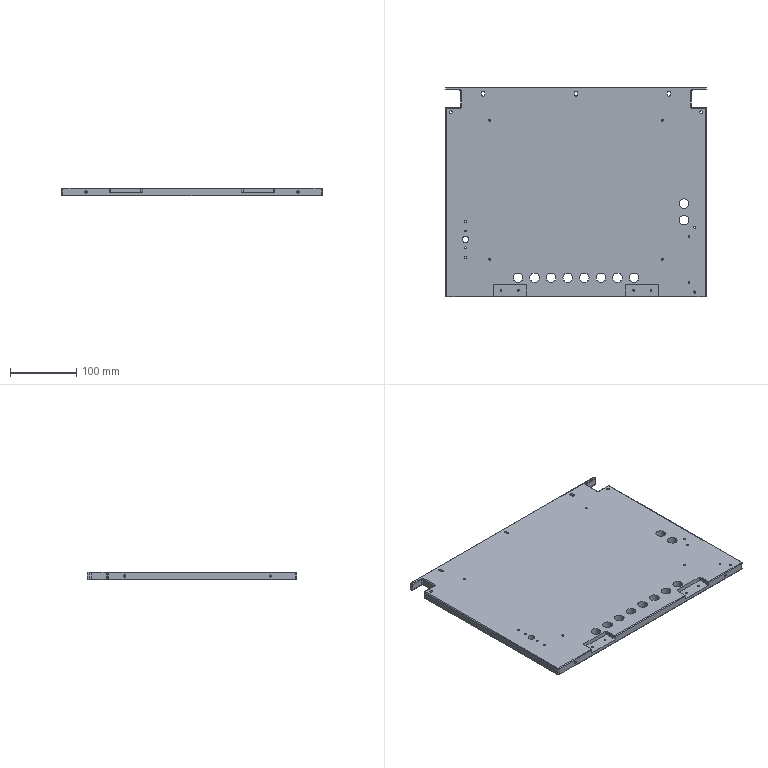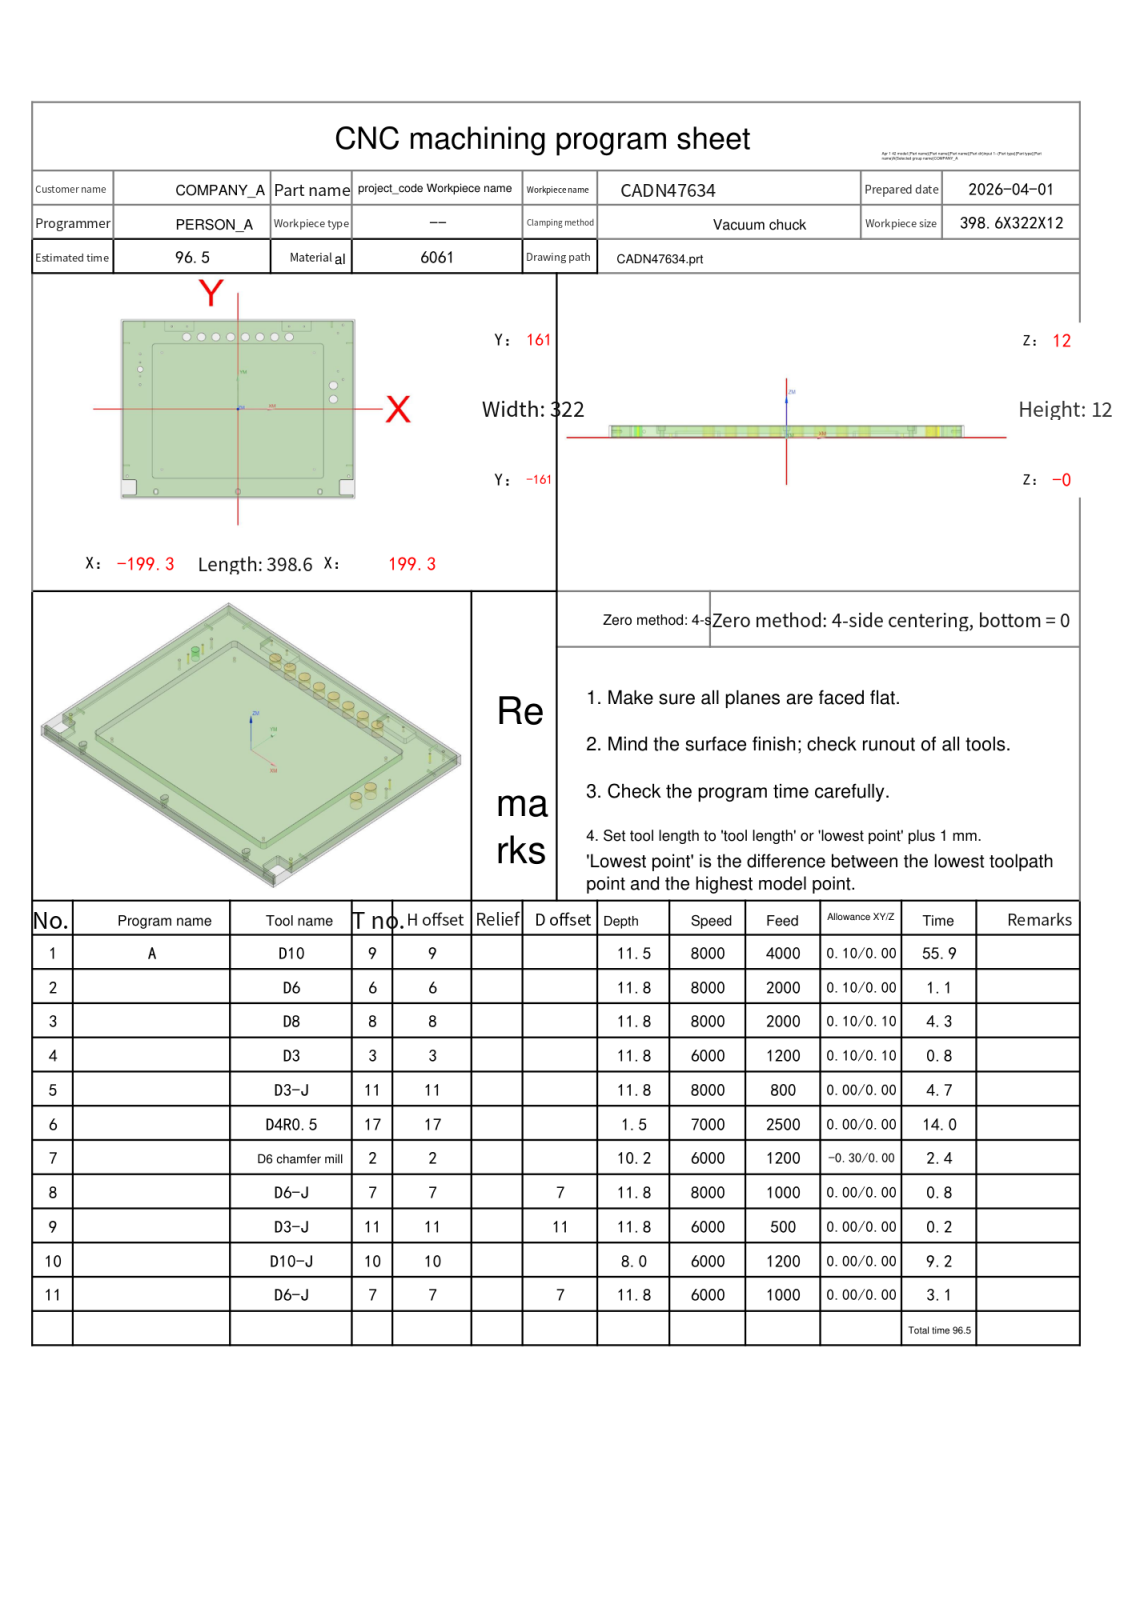NC program | NX | posted by the shop | part box 393.6 x 317 x 12 mm
Lines 1 to 3047 of 16012, first 2196 of 3045 lines:
%
O0001
(Machine time: 98.57 MIN)
(===Total Tool:9===)
(T9=D10     D=10.  R=0.   D-  H09 Z=0.5   )
(T6=D6      D=6.   R=0.   D-  H06 Z=0.2   )
(T8=D8      D=8.   R=0.   D-  H08 Z=0.2   )
(T3=D3      D=3.   R=0.   D-  H03 Z=0.2   )
(T11=D3-J   D=3.   R=0.   D-  H11 Z=0.2   )
(T17=D4R0.5 D=4.   R=0.5  D-  H17 Z=10.5  )
(T2=D6 chamfer mill   D=6.   R=0.   D-  H02 Z=1.8   )
(T7=D6-J    D=6.   R=0.   D7  H07 Z=0.2   )
(T10=D10-J  D=10.  R=0.   D10 H10 Z=4.    )
G80 G90 G17 G49 G40
G91 G28 Z0
M01
N1 T09 M06
(D10  D=10. R=0. H=09 ce=0.10 di=0.10)
G00 G90 G54 X-27.65 Y.4 M03 S8000
G43 H09 Z32.
M08
Z12.5
G01 X-28.9 Z12.467 F3500.
Y-7.4 Z12.263
X0.0 Z11.506
X28.9
Y.4
X-28.9
Y-7.4
X0.0
Y-14.4
X35.9
Y7.4
X-35.9
Y-14.4
X0.0
Y-21.4
X42.9
Y14.4
X-42.9
Y-21.4
X0.0
Y-28.4
X49.9
Y21.4
X-49.9
Y-28.4
X0.0
Y-35.4
X56.9
Y28.4
X-56.9
Y-35.4
X0.0
Y-42.4
X63.9
Y35.4
X-63.9
Y-42.4
X0.0
Y-49.4
X70.9
Y42.4
X-70.9
Y-49.4
X0.0
Y-56.4
X77.9
Y49.4
X-77.9
Y-56.4
X0.0
Y-63.4
X84.9
Y56.4
X-84.9
Y-63.4
X0.0
Y-70.4
X91.9
Y63.4
X-91.9
Y-70.4
X0.0
Y-77.4
X98.9
Y70.4
X-98.9
Y-77.4
X0.0
Y-84.4
X105.9
Y77.4
X-105.9
Y-84.4
X0.0
Y-91.4
X112.9
Y84.4
X-112.9
Y-91.4
X0.0
Y-98.4
X119.9
Y91.4
X-119.9
Y-98.4
X0.0
Y-105.4
X126.9
Y98.4
X-126.9
Y-105.4
X0.0
Y-112.4
X133.9
Y105.4
X-133.9
Y-112.4
X0.0
Y-119.4
X140.9
Y112.4
X-140.9
Y-119.4
X0.0
X.5
Z12.006
G00 Z12.5
X-27.65 Y.4
Z12.006
G01 X-28.9 Z11.974
Y-7.4 Z11.769
X0.0 Z11.013
X28.9
Y.4
X-28.9
Y-7.4
X0.0
Y-14.4
X35.9
Y7.4
X-35.9
Y-14.4
X0.0
Y-21.4
X42.9
Y14.4
X-42.9
Y-21.4
X0.0
Y-28.4
X49.9
Y21.4
X-49.9
Y-28.4
X0.0
Y-35.4
X56.9
Y28.4
X-56.9
Y-35.4
X0.0
Y-42.4
X63.9
Y35.4
X-63.9
Y-42.4
X0.0
Y-49.4
X70.9
Y42.4
X-70.9
Y-49.4
X0.0
Y-56.4
X77.9
Y49.4
X-77.9
Y-56.4
X0.0
Y-63.4
X84.9
Y56.4
X-84.9
Y-63.4
X0.0
Y-70.4
X91.9
Y63.4
X-91.9
Y-70.4
X0.0
Y-77.4
X98.9
Y70.4
X-98.9
Y-77.4
X0.0
Y-84.4
X105.9
Y77.4
X-105.9
Y-84.4
X0.0
Y-91.4
X112.9
Y84.4
X-112.9
Y-91.4
X0.0
Y-98.4
X119.9
Y91.4
X-119.9
Y-98.4
X0.0
Y-105.4
X126.9
Y98.4
X-126.9
Y-105.4
X0.0
Y-112.4
X133.9
Y105.4
X-133.9
Y-112.4
X0.0
Y-119.4
X140.9
Y112.4
X-140.9
Y-119.4
X0.0
X.5
Z11.513
G00 Z12.006
X-27.65 Y.4
Z11.513
G01 X-28.9 Z11.48
Y-7.4 Z11.276
X0.0 Z10.519
X28.9
Y.4
X-28.9
Y-7.4
X0.0
Y-14.4
X35.9
Y7.4
X-35.9
Y-14.4
X0.0
Y-21.4
X42.9
Y14.4
X-42.9
Y-21.4
X0.0
Y-28.4
X49.9
Y21.4
X-49.9
Y-28.4
X0.0
Y-35.4
X56.9
Y28.4
X-56.9
Y-35.4
X0.0
Y-42.4
X63.9
Y35.4
X-63.9
Y-42.4
X0.0
Y-49.4
X70.9
Y42.4
X-70.9
Y-49.4
X0.0
Y-56.4
X77.9
Y49.4
X-77.9
Y-56.4
X0.0
Y-63.4
X84.9
Y56.4
X-84.9
Y-63.4
X0.0
Y-70.4
X91.9
Y63.4
X-91.9
Y-70.4
X0.0
Y-77.4
X98.9
Y70.4
X-98.9
Y-77.4
X0.0
Y-84.4
X105.9
Y77.4
X-105.9
Y-84.4
X0.0
Y-91.4
X112.9
Y84.4
X-112.9
Y-91.4
X0.0
Y-98.4
X119.9
Y91.4
X-119.9
Y-98.4
X0.0
Y-105.4
X126.9
Y98.4
X-126.9
Y-105.4
X0.0
Y-112.4
X133.9
Y105.4
X-133.9
Y-112.4
X0.0
Y-119.4
X140.9
Y112.4
X-140.9
Y-119.4
X0.0
X.5
Z11.019
G00 Z11.513
X-27.65 Y.4
Z11.019
G01 X-28.9 Z10.986
Y-7.4 Z10.782
X0.0 Z10.025
X28.9
Y.4
X-28.9
Y-7.4
X0.0
Y-14.4
X35.9
Y7.4
X-35.9
Y-14.4
X0.0
Y-21.4
X42.9
Y14.4
X-42.9
Y-21.4
X0.0
Y-28.4
X49.9
Y21.4
X-49.9
Y-28.4
X0.0
Y-35.4
X56.9
Y28.4
X-56.9
Y-35.4
X0.0
Y-42.4
X63.9
Y35.4
X-63.9
Y-42.4
X0.0
Y-49.4
X70.9
Y42.4
X-70.9
Y-49.4
X0.0
Y-56.4
X77.9
Y49.4
X-77.9
Y-56.4
X0.0
Y-63.4
X84.9
Y56.4
X-84.9
Y-63.4
X0.0
Y-70.4
X91.9
Y63.4
X-91.9
Y-70.4
X0.0
Y-77.4
X98.9
Y70.4
X-98.9
Y-77.4
X0.0
Y-84.4
X105.9
Y77.4
X-105.9
Y-84.4
X0.0
Y-91.4
X112.9
Y84.4
X-112.9
Y-91.4
X0.0
Y-98.4
X119.9
Y91.4
X-119.9
Y-98.4
X0.0
Y-105.4
X126.9
Y98.4
X-126.9
Y-105.4
X0.0
Y-112.4
X133.9
Y105.4
X-133.9
Y-112.4
X0.0
Y-119.4
X140.9
Y112.4
X-140.9
Y-119.4
X0.0
X.5
Z10.525
G00 Z11.019
X-27.65 Y.4
Z10.525
G01 X-28.9 Z10.492
Y-7.4 Z10.288
X0.0 Z9.531
X28.9
Y.4
X-28.9
Y-7.4
X0.0
Y-14.4
X35.9
Y7.4
X-35.9
Y-14.4
X0.0
Y-21.4
X42.9
Y14.4
X-42.9
Y-21.4
X0.0
Y-28.4
X49.9
Y21.4
X-49.9
Y-28.4
X0.0
Y-35.4
X56.9
Y28.4
X-56.9
Y-35.4
X0.0
Y-42.4
X63.9
Y35.4
X-63.9
Y-42.4
X0.0
Y-49.4
X70.9
Y42.4
X-70.9
Y-49.4
X0.0
Y-56.4
X77.9
Y49.4
X-77.9
Y-56.4
X0.0
Y-63.4
X84.9
Y56.4
X-84.9
Y-63.4
X0.0
Y-70.4
X91.9
Y63.4
X-91.9
Y-70.4
X0.0
Y-77.4
X98.9
Y70.4
X-98.9
Y-77.4
X0.0
Y-84.4
X105.9
Y77.4
X-105.9
Y-84.4
X0.0
Y-91.4
X112.9
Y84.4
X-112.9
Y-91.4
X0.0
Y-98.4
X119.9
Y91.4
X-119.9
Y-98.4
X0.0
Y-105.4
X126.9
Y98.4
X-126.9
Y-105.4
X0.0
Y-112.4
X133.9
Y105.4
X-133.9
Y-112.4
X0.0
Y-119.4
X140.9
Y112.4
X-140.9
Y-119.4
X0.0
X.5
Z10.031
G00 Z10.525
X-27.65 Y.4
Z10.031
G01 X-28.9 Z9.999
Y-7.4 Z9.794
X0.0 Z9.038
X28.9
Y.4
X-28.9
Y-7.4
X0.0
Y-14.4
X35.9
Y7.4
X-35.9
Y-14.4
X0.0
Y-21.4
X42.9
Y14.4
X-42.9
Y-21.4
X0.0
Y-28.4
X49.9
Y21.4
X-49.9
Y-28.4
X0.0
Y-35.4
X56.9
Y28.4
X-56.9
Y-35.4
X0.0
Y-42.4
X63.9
Y35.4
X-63.9
Y-42.4
X0.0
Y-49.4
X70.9
Y42.4
X-70.9
Y-49.4
X0.0
Y-56.4
X77.9
Y49.4
X-77.9
Y-56.4
X0.0
Y-63.4
X84.9
Y56.4
X-84.9
Y-63.4
X0.0
Y-70.4
X91.9
Y63.4
X-91.9
Y-70.4
X0.0
Y-77.4
X98.9
Y70.4
X-98.9
Y-77.4
X0.0
Y-84.4
X105.9
Y77.4
X-105.9
Y-84.4
X0.0
Y-91.4
X112.9
Y84.4
X-112.9
Y-91.4
X0.0
Y-98.4
X119.9
Y91.4
X-119.9
Y-98.4
X0.0
Y-105.4
X126.9
Y98.4
X-126.9
Y-105.4
X0.0
Y-112.4
X133.9
Y105.4
X-133.9
Y-112.4
X0.0
Y-119.4
X140.9
Y112.4
X-140.9
Y-119.4
X0.0
X.5
Z9.538
G00 Z10.031
X-27.65 Y.4
Z9.538
G01 X-28.9 Z9.505
Y-7.4 Z9.301
X0.0 Z8.544
X28.9
Y.4
X-28.9
Y-7.4
X0.0
Y-14.4
X35.9
Y7.4
X-35.9
Y-14.4
X0.0
Y-21.4
X42.9
Y14.4
X-42.9
Y-21.4
X0.0
Y-28.4
X49.9
Y21.4
X-49.9
Y-28.4
X0.0
Y-35.4
X56.9
Y28.4
X-56.9
Y-35.4
X0.0
Y-42.4
X63.9
Y35.4
X-63.9
Y-42.4
X0.0
Y-49.4
X70.9
Y42.4
X-70.9
Y-49.4
X0.0
Y-56.4
X77.9
Y49.4
X-77.9
Y-56.4
X0.0
Y-63.4
X84.9
Y56.4
X-84.9
Y-63.4
X0.0
Y-70.4
X91.9
Y63.4
X-91.9
Y-70.4
X0.0
Y-77.4
X98.9
Y70.4
X-98.9
Y-77.4
X0.0
Y-84.4
X105.9
Y77.4
X-105.9
Y-84.4
X0.0
Y-91.4
X112.9
Y84.4
X-112.9
Y-91.4
X0.0
Y-98.4
X119.9
Y91.4
X-119.9
Y-98.4
X0.0
Y-105.4
X126.9
Y98.4
X-126.9
Y-105.4
X0.0
Y-112.4
X133.9
Y105.4
X-133.9
Y-112.4
X0.0
Y-119.4
X140.9
Y112.4
X-140.9
Y-119.4
X0.0
X.5
Z9.044
G00 Z9.538
X-27.65 Y.4
Z9.044
G01 X-28.9 Z9.011
Y-7.4 Z8.807
X0.0 Z8.05
X28.9
Y.4
X-28.9
Y-7.4
X0.0
Y-14.4
X35.9
Y7.4
X-35.9
Y-14.4
X0.0
Y-21.4
X42.9
Y14.4
X-42.9
Y-21.4
X0.0
Y-28.4
X49.9
Y21.4
X-49.9
Y-28.4
X0.0
Y-35.4
X56.9
Y28.4
X-56.9
Y-35.4
X0.0
Y-42.4
X63.9
Y35.4
X-63.9
Y-42.4
X0.0
Y-49.4
X70.9
Y42.4
X-70.9
Y-49.4
X0.0
Y-56.4
X77.9
Y49.4
X-77.9
Y-56.4
X0.0
Y-63.4
X84.9
Y56.4
X-84.9
Y-63.4
X0.0
Y-70.4
X91.9
Y63.4
X-91.9
Y-70.4
X0.0
Y-77.4
X98.9
Y70.4
X-98.9
Y-77.4
X0.0
Y-84.4
X105.9
Y77.4
X-105.9
Y-84.4
X0.0
Y-91.4
X112.9
Y84.4
X-112.9
Y-91.4
X0.0
Y-98.4
X119.9
Y91.4
X-119.9
Y-98.4
X0.0
Y-105.4
X126.9
Y98.4
X-126.9
Y-105.4
X0.0
Y-112.4
X133.9
Y105.4
X-133.9
Y-112.4
X0.0
Y-119.4
X140.9
Y112.4
X-140.9
Y-119.4
X0.0
X.5
Z8.55
G00 Z9.044
X-27.65 Y.4
Z8.55
G01 X-28.9 Z8.517
Y-7.4 Z8.313
X0.0 Z7.556
X28.9
Y.4
X-28.9
Y-7.4
X0.0
Y-14.4
X35.9
Y7.4
X-35.9
Y-14.4
X0.0
Y-21.4
X42.9
Y14.4
X-42.9
Y-21.4
X0.0
Y-28.4
X49.9
Y21.4
X-49.9
Y-28.4
X0.0
Y-35.4
X56.9
Y28.4
X-56.9
Y-35.4
X0.0
Y-42.4
X63.9
Y35.4
X-63.9
Y-42.4
X0.0
Y-49.4
X70.9
Y42.4
X-70.9
Y-49.4
X0.0
Y-56.4
X77.9
Y49.4
X-77.9
Y-56.4
X0.0
Y-63.4
X84.9
Y56.4
X-84.9
Y-63.4
X0.0
Y-70.4
X91.9
Y63.4
X-91.9
Y-70.4
X0.0
Y-77.4
X98.9
Y70.4
X-98.9
Y-77.4
X0.0
Y-84.4
X105.9
Y77.4
X-105.9
Y-84.4
X0.0
Y-91.4
X112.9
Y84.4
X-112.9
Y-91.4
X0.0
Y-98.4
X119.9
Y91.4
X-119.9
Y-98.4
X0.0
Y-105.4
X126.9
Y98.4
X-126.9
Y-105.4
X0.0
Y-112.4
X133.9
Y105.4
X-133.9
Y-112.4
X0.0
Y-119.4
X140.9
Y112.4
X-140.9
Y-119.4
X0.0
X.5
Z8.056
G00 Z8.55
X-27.65 Y.4
Z8.056
G01 X-28.9 Z8.024
Y-7.4 Z7.819
X0.0 Z7.063
X28.9
Y.4
X-28.9
Y-7.4
X0.0
Y-14.4
X35.9
Y7.4
X-35.9
Y-14.4
X0.0
Y-21.4
X42.9
Y14.4
X-42.9
Y-21.4
X0.0
Y-28.4
X49.9
Y21.4
X-49.9
Y-28.4
X0.0
Y-35.4
X56.9
Y28.4
X-56.9
Y-35.4
X0.0
Y-42.4
X63.9
Y35.4
X-63.9
Y-42.4
X0.0
Y-49.4
X70.9
Y42.4
X-70.9
Y-49.4
X0.0
Y-56.4
X77.9
Y49.4
X-77.9
Y-56.4
X0.0
Y-63.4
X84.9
Y56.4
X-84.9
Y-63.4
X0.0
Y-70.4
X91.9
Y63.4
X-91.9
Y-70.4
X0.0
Y-77.4
X98.9
Y70.4
X-98.9
Y-77.4
X0.0
Y-84.4
X105.9
Y77.4
X-105.9
Y-84.4
X0.0
Y-91.4
X112.9
Y84.4
X-112.9
Y-91.4
X0.0
Y-98.4
X119.9
Y91.4
X-119.9
Y-98.4
X0.0
Y-105.4
X126.9
Y98.4
X-126.9
Y-105.4
X0.0
Y-112.4
X133.9
Y105.4
X-133.9
Y-112.4
X0.0
Y-119.4
X140.9
Y112.4
X-140.9
Y-119.4
X0.0
X.5
Z7.563
G00 Z8.056
X-27.65 Y.4
Z7.563
G01 X-28.9 Z7.53
Y-7.4 Z7.326
X0.0 Z6.569
X28.9
Y.4
X-28.9
Y-7.4
X0.0
Y-14.4
X35.9
Y7.4
X-35.9
Y-14.4
X0.0
Y-21.4
X42.9
Y14.4
X-42.9
Y-21.4
X0.0
Y-28.4
X49.9
Y21.4
X-49.9
Y-28.4
X0.0
Y-35.4
X56.9
Y28.4
X-56.9
Y-35.4
X0.0
Y-42.4
X63.9
Y35.4
X-63.9
Y-42.4
X0.0
Y-49.4
X70.9
Y42.4
X-70.9
Y-49.4
X0.0
Y-56.4
X77.9
Y49.4
X-77.9
Y-56.4
X0.0
Y-63.4
X84.9
Y56.4
X-84.9
Y-63.4
X0.0
Y-70.4
X91.9
Y63.4
X-91.9
Y-70.4
X0.0
Y-77.4
X98.9
Y70.4
X-98.9
Y-77.4
X0.0
Y-84.4
X105.9
Y77.4
X-105.9
Y-84.4
X0.0
Y-91.4
X112.9
Y84.4
X-112.9
Y-91.4
X0.0
Y-98.4
X119.9
Y91.4
X-119.9
Y-98.4
X0.0
Y-105.4
X126.9
Y98.4
X-126.9
Y-105.4
X0.0
Y-112.4
X133.9
Y105.4
X-133.9
Y-112.4
X0.0
Y-119.4
X140.9
Y112.4
X-140.9
Y-119.4
X0.0
X.5
Z7.069
G00 Z7.563
X-27.65 Y.4
Z7.069
G01 X-28.9 Z7.036
Y-7.4 Z6.832
X0.0 Z6.075
X28.9
Y.4
X-28.9
Y-7.4
X0.0
Y-14.4
X35.9
Y7.4
X-35.9
Y-14.4
X0.0
Y-21.4
X42.9
Y14.4
X-42.9
Y-21.4
X0.0
Y-28.4
X49.9
Y21.4
X-49.9
Y-28.4
X0.0
Y-35.4
X56.9
Y28.4
X-56.9
Y-35.4
X0.0
Y-42.4
X63.9
Y35.4
X-63.9
Y-42.4
X0.0
Y-49.4
X70.9
Y42.4
X-70.9
Y-49.4
X0.0
Y-56.4
X77.9
Y49.4
X-77.9
Y-56.4
X0.0
Y-63.4
X84.9
Y56.4
X-84.9
Y-63.4
X0.0
Y-70.4
X91.9
Y63.4
X-91.9
Y-70.4
X0.0
Y-77.4
X98.9
Y70.4
X-98.9
Y-77.4
X0.0
Y-84.4
X105.9
Y77.4
X-105.9
Y-84.4
X0.0
Y-91.4
X112.9
Y84.4
X-112.9
Y-91.4
X0.0
Y-98.4
X119.9
Y91.4
X-119.9
Y-98.4
X0.0
Y-105.4
X126.9
Y98.4
X-126.9
Y-105.4
X0.0
Y-112.4
X133.9
Y105.4
X-133.9
Y-112.4
X0.0
Y-119.4
X140.9
Y112.4
X-140.9
Y-119.4
X0.0
X.5
Z6.575
G00 Z7.069
X-27.65 Y.4
Z6.575
G01 X-28.9 Z6.542
Y-7.4 Z6.338
X0.0 Z5.581
X28.9
Y.4
X-28.9
Y-7.4
X0.0
Y-14.4
X35.9
Y7.4
X-35.9
Y-14.4
X0.0
Y-21.4
X42.9
Y14.4
X-42.9
Y-21.4
X0.0
Y-28.4
X49.9
Y21.4
X-49.9
Y-28.4
X0.0
Y-35.4
X56.9
Y28.4
X-56.9
Y-35.4
X0.0
Y-42.4
X63.9
Y35.4
X-63.9
Y-42.4
X0.0
Y-49.4
X70.9
Y42.4
X-70.9
Y-49.4
X0.0
Y-56.4
X77.9
Y49.4
X-77.9
Y-56.4
X0.0
Y-63.4
X84.9
Y56.4
X-84.9
Y-63.4
X0.0
Y-70.4
X91.9
Y63.4
X-91.9
Y-70.4
X0.0
Y-77.4
X98.9
Y70.4
X-98.9
Y-77.4
X0.0
Y-84.4
X105.9
Y77.4
X-105.9
Y-84.4
X0.0
Y-91.4
X112.9
Y84.4
X-112.9
Y-91.4
X0.0
Y-98.4
X119.9
Y91.4
X-119.9
Y-98.4
X0.0
Y-105.4
X126.9
Y98.4
X-126.9
Y-105.4
X0.0
Y-112.4
X133.9
Y105.4
X-133.9
Y-112.4
X0.0
Y-119.4
X140.9
Y112.4
X-140.9
Y-119.4
X0.0
X.5
Z6.081
G00 Z6.575
X-27.65 Y.4
Z6.081
G01 X-28.9 Z6.049
Y-7.4 Z5.844
X0.0 Z5.088
X28.9
Y.4
X-28.9
Y-7.4
X0.0
Y-14.4
X35.9
Y7.4
X-35.9
Y-14.4
X0.0
Y-21.4
X42.9
Y14.4
X-42.9
Y-21.4
X0.0
Y-28.4
X49.9
Y21.4
X-49.9
Y-28.4
X0.0
Y-35.4
X56.9
Y28.4
X-56.9
Y-35.4
X0.0
Y-42.4
X63.9
Y35.4
X-63.9
Y-42.4
X0.0
Y-49.4
X70.9
Y42.4
X-70.9
Y-49.4
X0.0
Y-56.4
X77.9
Y49.4
X-77.9
Y-56.4
X0.0
Y-63.4
X84.9
Y56.4
X-84.9
Y-63.4
X0.0
Y-70.4
X91.9
Y63.4
X-91.9
Y-70.4
X0.0
Y-77.4
X98.9
Y70.4
X-98.9
Y-77.4
X0.0
Y-84.4
X105.9
Y77.4
X-105.9
Y-84.4
X0.0
Y-91.4
X112.9
Y84.4
X-112.9
Y-91.4
X0.0
Y-98.4
X119.9
Y91.4
X-119.9
Y-98.4
X0.0
Y-105.4
X126.9
Y98.4
X-126.9
Y-105.4
X0.0
Y-112.4
X133.9
Y105.4
X-133.9
Y-112.4
X0.0
Y-119.4
X140.9
Y112.4
X-140.9
Y-119.4
X0.0
X.5
Z5.588
G00 Z6.081
X-27.65 Y.4
Z5.588
G01 X-28.9 Z5.555
Y-7.4 Z5.351
X0.0 Z4.594
X28.9
Y.4
X-28.9
Y-7.4
X0.0
Y-14.4
X35.9
Y7.4
X-35.9
Y-14.4
X0.0
Y-21.4
X42.9
Y14.4
X-42.9
Y-21.4
X0.0
Y-28.4
X49.9
Y21.4
X-49.9
Y-28.4
X0.0
Y-35.4
X56.9
Y28.4
X-56.9
Y-35.4
X0.0
Y-42.4
X63.9
Y35.4
X-63.9
Y-42.4
X0.0
Y-49.4
X70.9
Y42.4
X-70.9
Y-49.4
X0.0
Y-56.4
X77.9
Y49.4
X-77.9
Y-56.4
X0.0
Y-63.4
X84.9
Y56.4
X-84.9
Y-63.4
X0.0
Y-70.4
X91.9
Y63.4
X-91.9
Y-70.4
X0.0
Y-77.4
X98.9
Y70.4
X-98.9
Y-77.4
X0.0
Y-84.4
X105.9
Y77.4
X-105.9
Y-84.4
X0.0
Y-91.4
X112.9
Y84.4
X-112.9
Y-91.4
X0.0
Y-98.4
X119.9
Y91.4
X-119.9
Y-98.4
X0.0
Y-105.4
X126.9
Y98.4
X-126.9
Y-105.4
X0.0
Y-112.4
X133.9
Y105.4
X-133.9
Y-112.4
X0.0
Y-119.4
X140.9
Y112.4
X-140.9
Y-119.4
X0.0
X.5
Z5.094
G00 Z5.588
X-27.65 Y.4
Z5.094
G01 X-28.9 Z5.061
Y-7.4 Z4.857
X0.0 Z4.1
X28.9
Y.4
X-28.9
Y-7.4
X0.0
Y-14.4
X35.9
Y7.4
X-35.9
Y-14.4
X0.0
Y-21.4
X42.9
Y14.4
X-42.9
Y-21.4
X0.0
Y-28.4
X49.9
Y21.4
X-49.9
Y-28.4
X0.0
Y-35.4
X56.9
Y28.4
X-56.9
Y-35.4
X0.0
Y-42.4
X63.9
Y35.4
X-63.9
Y-42.4
X0.0
Y-49.4
X70.9
Y42.4
X-70.9
Y-49.4
X0.0
Y-56.4
X77.9
Y49.4
X-77.9
Y-56.4
X0.0
Y-63.4
X84.9
Y56.4
X-84.9
Y-63.4
X0.0
Y-70.4
X91.9
Y63.4
X-91.9
Y-70.4
X0.0
Y-77.4
X98.9
Y70.4
X-98.9
Y-77.4
X0.0
Y-84.4
X105.9
Y77.4
X-105.9
Y-84.4
X0.0
Y-91.4
X112.9
Y84.4
X-112.9
Y-91.4
X0.0
Y-98.4
X119.9
Y91.4
X-119.9
Y-98.4
X0.0
Y-105.4
X126.9
Y98.4
X-126.9
Y-105.4
X0.0
Y-112.4
X133.9
Y105.4
X-133.9
Y-112.4
X0.0
Y-119.4
X140.9
Y112.4
X-140.9
Y-119.4
X0.0
X.5
Z4.6
G00 Z32.
G00 G90 X0.0 Y-163.6 M03 S6000
Z32.
Z12.5
G01 X-195.8 Z12.439 F4000.
G02 X-201.9 Y-157.5 Z12.436 I0.0 J6.1
G01 Y-155.001 Z12.435
G02 X-195.8 Y-148.901 Z12.432 I6.1 J0.0
G01 X-179. Y-148.9 Z12.427
Y-132.6 Z12.421
X-195.8 Z12.416
G02 X-201.9 Y-126.5 Z12.413 I0.0 J6.1
G01 Y156.5 Z12.325
G02 X-194.8 Y163.6 Z12.321 I7.1 J0.0
G01 X194.8 Z12.199
G02 X201.9 Y156.5 Z12.195 I0.0 J-7.1
G01 Y-126.5 Z12.107
G02 X195.8 Y-132.6 Z12.104 I-6.1 J0.0
G01 X179. Z12.099
Y-148.9 Z12.093
X195.8 Y-148.901 Z12.088
G02 X201.9 Y-155.001 Z12.085 I0.0 J-6.1
G01 Y-157.5 Z12.084
G02 X195.8 Y-163.6 Z12.081 I-6.1 J0.0
G01 X-195.8 Z11.959
G02 X-201.9 Y-157.5 Z11.956 I0.0 J6.1
G01 Y-155.001 Z11.955
G02 X-195.8 Y-148.901 Z11.952 I6.1 J0.0
G01 X-179. Y-148.9 Z11.947
Y-132.6 Z11.941
X-195.8 Z11.936
G02 X-201.9 Y-126.5 Z11.933 I0.0 J6.1
G01 Y156.5 Z11.845
G02 X-194.8 Y163.6 Z11.841 I7.1 J0.0
G01 X194.8 Z11.719
G02 X201.9 Y156.5 Z11.715 I0.0 J-7.1
G01 Y-126.5 Z11.627
G02 X195.8 Y-132.6 Z11.624 I-6.1 J0.0
G01 X179. Z11.619
Y-148.9 Z11.613
X195.8 Y-148.901 Z11.608
G02 X201.9 Y-155.001 Z11.605 I0.0 J-6.1
G01 Y-157.5 Z11.604
G02 X195.8 Y-163.6 Z11.601 I-6.1 J0.0
G01 X-195.8 Z11.479
G02 X-201.9 Y-157.5 Z11.476 I0.0 J6.1
G01 Y-155.001 Z11.475
G02 X-195.8 Y-148.901 Z11.472 I6.1 J0.0
G01 X-179. Y-148.9 Z11.467
Y-132.6 Z11.461
X-195.8 Z11.456
G02 X-201.9 Y-126.5 Z11.453 I0.0 J6.1
G01 Y156.5 Z11.365
G02 X-194.8 Y163.6 Z11.361 I7.1 J0.0
G01 X194.8 Z11.239
G02 X201.9 Y156.5 Z11.235 I0.0 J-7.1
G01 Y-126.5 Z11.147
G02 X195.8 Y-132.6 Z11.144 I-6.1 J0.0
G01 X179. Z11.139
Y-148.9 Z11.133
X195.8 Y-148.901 Z11.128
G02 X201.9 Y-155.001 Z11.125 I0.0 J-6.1
G01 Y-157.5 Z11.124
G02 X195.8 Y-163.6 Z11.121 I-6.1 J0.0
G01 X-195.8 Z10.999
G02 X-201.9 Y-157.5 Z10.996 I0.0 J6.1
G01 Y-155.001 Z10.995
G02 X-195.8 Y-148.901 Z10.992 I6.1 J0.0
G01 X-179. Y-148.9 Z10.987
Y-132.6 Z10.981
X-195.8 Z10.976
G02 X-201.9 Y-126.5 Z10.973 I0.0 J6.1
G01 Y156.5 Z10.885
G02 X-194.8 Y163.6 Z10.881 I7.1 J0.0
G01 X194.8 Z10.759
G02 X201.9 Y156.5 Z10.755 I0.0 J-7.1
G01 Y-126.5 Z10.667
G02 X195.8 Y-132.6 Z10.664 I-6.1 J0.0
G01 X179. Z10.659
Y-148.9 Z10.653
X195.8 Y-148.901 Z10.648
G02 X201.9 Y-155.001 Z10.645 I0.0 J-6.1
G01 Y-157.5 Z10.644
G02 X195.8 Y-163.6 Z10.641 I-6.1 J0.0
G01 X-195.8 Z10.519
G02 X-201.9 Y-157.5 Z10.516 I0.0 J6.1
G01 Y-155.001 Z10.515
G02 X-195.8 Y-148.901 Z10.512 I6.1 J0.0
G01 X-179. Y-148.9 Z10.507
Y-132.6 Z10.501
X-195.8 Z10.496
G02 X-201.9 Y-126.5 Z10.493 I0.0 J6.1
G01 Y156.5 Z10.405
G02 X-194.8 Y163.6 Z10.401 I7.1 J0.0
G01 X194.8 Z10.279
G02 X201.9 Y156.5 Z10.275 I0.0 J-7.1
G01 Y-126.5 Z10.187
G02 X195.8 Y-132.6 Z10.184 I-6.1 J0.0
G01 X179. Z10.179
Y-148.9 Z10.173
X195.8 Y-148.901 Z10.168
G02 X201.9 Y-155.001 Z10.165 I0.0 J-6.1
G01 Y-157.5 Z10.164
G02 X195.8 Y-163.6 Z10.161 I-6.1 J0.0
G01 X-195.8 Z10.039
G02 X-201.9 Y-157.5 Z10.036 I0.0 J6.1
G01 Y-155.001 Z10.035
G02 X-195.8 Y-148.901 Z10.032 I6.1 J0.0
G01 X-179. Y-148.9 Z10.027
Y-132.6 Z10.021
X-195.8 Z10.016
G02 X-201.9 Y-126.5 Z10.013 I0.0 J6.1
G01 Y156.5 Z9.925
G02 X-194.8 Y163.6 Z9.921 I7.1 J0.0
G01 X194.8 Z9.799
G02 X201.9 Y156.5 Z9.795 I0.0 J-7.1
G01 Y-126.5 Z9.707
G02 X195.8 Y-132.6 Z9.704 I-6.1 J0.0
G01 X179. Z9.699
Y-148.9 Z9.693
X195.8 Y-148.901 Z9.688
G02 X201.9 Y-155.001 Z9.685 I0.0 J-6.1
G01 Y-157.5 Z9.684
G02 X195.8 Y-163.6 Z9.681 I-6.1 J0.0
G01 X-195.8 Z9.559
G02 X-201.9 Y-157.5 Z9.556 I0.0 J6.1
G01 Y-155.001 Z9.555
G02 X-195.8 Y-148.901 Z9.552 I6.1 J0.0
G01 X-179. Y-148.9 Z9.547
Y-132.6 Z9.541
X-195.8 Z9.536
G02 X-201.9 Y-126.5 Z9.533 I0.0 J6.1
G01 Y156.5 Z9.445
G02 X-194.8 Y163.6 Z9.441 I7.1 J0.0
G01 X194.8 Z9.319
G02 X201.9 Y156.5 Z9.315 I0.0 J-7.1
G01 Y-126.5 Z9.227
G02 X195.8 Y-132.6 Z9.224 I-6.1 J0.0
G01 X179. Z9.219
Y-148.9 Z9.213
X195.8 Y-148.901 Z9.208
G02 X201.9 Y-155.001 Z9.205 I0.0 J-6.1
G01 Y-157.5 Z9.204
G02 X195.8 Y-163.6 Z9.201 I-6.1 J0.0
G01 X-195.8 Z9.079
G02 X-201.9 Y-157.5 Z9.076 I0.0 J6.1
G01 Y-155.001 Z9.075
G02 X-195.8 Y-148.901 Z9.072 I6.1 J0.0
G01 X-179. Y-148.9 Z9.067
Y-132.6 Z9.061
X-195.8 Z9.056
G02 X-201.9 Y-126.5 Z9.053 I0.0 J6.1
G01 Y156.5 Z8.965
G02 X-194.8 Y163.6 Z8.961 I7.1 J0.0
G01 X194.8 Z8.839
G02 X201.9 Y156.5 Z8.835 I0.0 J-7.1
G01 Y-126.5 Z8.747
G02 X195.8 Y-132.6 Z8.744 I-6.1 J0.0
G01 X179. Z8.739
Y-148.9 Z8.733
X195.8 Y-148.901 Z8.728
G02 X201.9 Y-155.001 Z8.725 I0.0 J-6.1
G01 Y-157.5 Z8.724
G02 X195.8 Y-163.6 Z8.721 I-6.1 J0.0
G01 X-195.8 Z8.599
G02 X-201.9 Y-157.5 Z8.596 I0.0 J6.1
G01 Y-155.001 Z8.595
G02 X-195.8 Y-148.901 Z8.592 I6.1 J0.0
G01 X-179. Y-148.9 Z8.587
Y-132.6 Z8.581
X-195.8 Z8.576
G02 X-201.9 Y-126.5 Z8.573 I0.0 J6.1
G01 Y156.5 Z8.485
G02 X-194.8 Y163.6 Z8.481 I7.1 J0.0
G01 X194.8 Z8.359
G02 X201.9 Y156.5 Z8.355 I0.0 J-7.1
G01 Y-126.5 Z8.267
G02 X195.8 Y-132.6 Z8.264 I-6.1 J0.0
G01 X179. Z8.259
Y-148.9 Z8.253
X195.8 Y-148.901 Z8.248
G02 X201.9 Y-155.001 Z8.245 I0.0 J-6.1
G01 Y-157.5 Z8.244
G02 X195.8 Y-163.6 Z8.241 I-6.1 J0.0
G01 X-195.8 Z8.119
G02 X-201.9 Y-157.5 Z8.116 I0.0 J6.1
G01 Y-155.001 Z8.115
G02 X-195.8 Y-148.901 Z8.112 I6.1 J0.0
G01 X-179. Y-148.9 Z8.107
Y-132.6 Z8.101
X-195.8 Z8.096
G02 X-201.9 Y-126.5 Z8.093 I0.0 J6.1
G01 Y156.5 Z8.005
G02 X-194.8 Y163.6 Z8.001 I7.1 J0.0
G01 X194.8 Z7.879
G02 X201.9 Y156.5 Z7.875 I0.0 J-7.1
G01 Y-126.5 Z7.787
G02 X195.8 Y-132.6 Z7.784 I-6.1 J0.0
G01 X179. Z7.779
Y-148.9 Z7.773
X195.8 Y-148.901 Z7.768
G02 X201.9 Y-155.001 Z7.765 I0.0 J-6.1
G01 Y-157.5 Z7.764
G02 X195.8 Y-163.6 Z7.761 I-6.1 J0.0
G01 X-195.8 Z7.639
G02 X-201.9 Y-157.5 Z7.636 I0.0 J6.1
G01 Y-155.001 Z7.635
G02 X-195.8 Y-148.901 Z7.632 I6.1 J0.0
G01 X-179. Y-148.9 Z7.627
Y-132.6 Z7.621
X-195.8 Z7.616
G02 X-201.9 Y-126.5 Z7.613 I0.0 J6.1
G01 Y156.5 Z7.525
G02 X-194.8 Y163.6 Z7.521 I7.1 J0.0
G01 X194.8 Z7.399
G02 X201.9 Y156.5 Z7.395 I0.0 J-7.1
G01 Y-126.5 Z7.307
G02 X195.8 Y-132.6 Z7.304 I-6.1 J0.0
G01 X179. Z7.299
Y-148.9 Z7.293
X195.8 Y-148.901 Z7.288
G02 X201.9 Y-155.001 Z7.285 I0.0 J-6.1
G01 Y-157.5 Z7.284
G02 X195.8 Y-163.6 Z7.281 I-6.1 J0.0
G01 X-195.8 Z7.159
G02 X-201.9 Y-157.5 Z7.156 I0.0 J6.1
G01 Y-155.001 Z7.155
G02 X-195.8 Y-148.901 Z7.152 I6.1 J0.0
G01 X-179. Y-148.9 Z7.147
Y-132.6 Z7.141
X-195.8 Z7.136
G02 X-201.9 Y-126.5 Z7.133 I0.0 J6.1
G01 Y156.5 Z7.045
G02 X-194.8 Y163.6 Z7.041 I7.1 J0.0
G01 X194.8 Z6.919
G02 X201.9 Y156.5 Z6.915 I0.0 J-7.1
G01 Y-126.5 Z6.827
G02 X195.8 Y-132.6 Z6.824 I-6.1 J0.0
G01 X179. Z6.819
Y-148.9 Z6.813
X195.8 Y-148.901 Z6.808
G02 X201.9 Y-155.001 Z6.805 I0.0 J-6.1
G01 Y-157.5 Z6.804
G02 X195.8 Y-163.6 Z6.801 I-6.1 J0.0
G01 X-195.8 Z6.679
G02 X-201.9 Y-157.5 Z6.676 I0.0 J6.1
G01 Y-155.001 Z6.675
G02 X-195.8 Y-148.901 Z6.672 I6.1 J0.0
G01 X-179. Y-148.9 Z6.667
Y-132.6 Z6.661
X-195.8 Z6.656
G02 X-201.9 Y-126.5 Z6.653 I0.0 J6.1
G01 Y156.5 Z6.565
G02 X-194.8 Y163.6 Z6.561 I7.1 J0.0
G01 X194.8 Z6.439
G02 X201.9 Y156.5 Z6.435 I0.0 J-7.1
G01 Y-126.5 Z6.347
G02 X195.8 Y-132.6 Z6.344 I-6.1 J0.0
G01 X179. Z6.339
Y-148.9 Z6.333
X195.8 Y-148.901 Z6.328
G02 X201.9 Y-155.001 Z6.325 I0.0 J-6.1
G01 Y-157.5 Z6.324
G02 X195.8 Y-163.6 Z6.321 I-6.1 J0.0
G01 X-195.8 Z6.199
G02 X-201.9 Y-157.5 Z6.196 I0.0 J6.1
G01 Y-155.001 Z6.195
G02 X-195.8 Y-148.901 Z6.192 I6.1 J0.0
G01 X-179. Y-148.9 Z6.187
Y-132.6 Z6.181
X-195.8 Z6.176
G02 X-201.9 Y-126.5 Z6.173 I0.0 J6.1
G01 Y156.5 Z6.085
G02 X-194.8 Y163.6 Z6.081 I7.1 J0.0
G01 X194.8 Z5.959
G02 X201.9 Y156.5 Z5.955 I0.0 J-7.1
G01 Y-126.5 Z5.867
G02 X195.8 Y-132.6 Z5.864 I-6.1 J0.0
G01 X179. Z5.859
Y-148.9 Z5.853
X195.8 Y-148.901 Z5.848
G02 X201.9 Y-155.001 Z5.845 I0.0 J-6.1
G01 Y-157.5 Z5.844
G02 X195.8 Y-163.6 Z5.841 I-6.1 J0.0
G01 X-195.8 Z5.719
G02 X-201.9 Y-157.5 Z5.716 I0.0 J6.1
G01 Y-155.001 Z5.715
G02 X-195.8 Y-148.901 Z5.712 I6.1 J0.0
G01 X-179. Y-148.9 Z5.707
Y-132.6 Z5.701
X-195.8 Z5.696
G02 X-201.9 Y-126.5 Z5.693 I0.0 J6.1
G01 Y156.5 Z5.605
G02 X-194.8 Y163.6 Z5.601 I7.1 J0.0
G01 X194.8 Z5.479
G02 X201.9 Y156.5 Z5.475 I0.0 J-7.1
G01 Y-126.5 Z5.387
G02 X195.8 Y-132.6 Z5.384 I-6.1 J0.0
G01 X179. Z5.379
Y-148.9 Z5.373
X195.8 Y-148.901 Z5.368
G02 X201.9 Y-155.001 Z5.365 I0.0 J-6.1
G01 Y-157.5 Z5.364
G02 X195.8 Y-163.6 Z5.361 I-6.1 J0.0
G01 X-195.8 Z5.239
G02 X-201.9 Y-157.5 Z5.236 I0.0 J6.1
G01 Y-155.001 Z5.235
G02 X-195.8 Y-148.901 Z5.232 I6.1 J0.0
G01 X-179. Y-148.9 Z5.227
Y-132.6 Z5.221
X-195.8 Z5.216
G02 X-201.9 Y-126.5 Z5.213 I0.0 J6.1
G01 Y156.5 Z5.125
G02 X-194.8 Y163.6 Z5.121 I7.1 J0.0
G01 X194.8 Z4.999
G02 X201.9 Y156.5 Z4.995 I0.0 J-7.1
G01 Y-126.5 Z4.907
G02 X195.8 Y-132.6 Z4.904 I-6.1 J0.0
G01 X179. Z4.899
Y-148.9 Z4.893
X195.8 Y-148.901 Z4.888
G02 X201.9 Y-155.001 Z4.885 I0.0 J-6.1
G01 Y-157.5 Z4.884
G02 X195.8 Y-163.6 Z4.881 I-6.1 J0.0
G01 X-195.8 Z4.759
G02 X-201.9 Y-157.5 Z4.756 I0.0 J6.1
G01 Y-155.001 Z4.755
G02 X-195.8 Y-148.901 Z4.752 I6.1 J0.0
G01 X-179. Y-148.9 Z4.747
Y-132.6 Z4.741
X-195.8 Z4.736
G02 X-201.9 Y-126.5 Z4.733 I0.0 J6.1
G01 Y156.5 Z4.645
G02 X-194.8 Y163.6 Z4.641 I7.1 J0.0
G01 X194.8 Z4.519
G02 X201.9 Y156.5 Z4.515 I0.0 J-7.1
G01 Y-126.5 Z4.427
G02 X195.8 Y-132.6 Z4.424 I-6.1 J0.0
G01 X179. Z4.419
Y-148.9 Z4.413
X195.8 Y-148.901 Z4.408
G02 X201.9 Y-155.001 Z4.405 I0.0 J-6.1
G01 Y-157.5 Z4.404
G02 X195.8 Y-163.6 Z4.401 I-6.1 J0.0
G01 X-195.8 Z4.279
G02 X-201.9 Y-157.5 Z4.276 I0.0 J6.1
G01 Y-155.001 Z4.275
G02 X-195.8 Y-148.901 Z4.272 I6.1 J0.0
G01 X-179. Y-148.9 Z4.267
Y-132.6 Z4.261
X-195.8 Z4.256
G02 X-201.9 Y-126.5 Z4.253 I0.0 J6.1
G01 Y156.5 Z4.165
G02 X-194.8 Y163.6 Z4.161 I7.1 J0.0
G01 X194.8 Z4.039
G02 X201.9 Y156.5 Z4.035 I0.0 J-7.1
G01 Y-126.5 Z3.947
G02 X195.8 Y-132.6 Z3.944 I-6.1 J0.0
G01 X179. Z3.939
Y-148.9 Z3.933
X195.8 Y-148.901 Z3.928
G02 X201.9 Y-155.001 Z3.925 I0.0 J-6.1
G01 Y-157.5 Z3.924
G02 X195.8 Y-163.6 Z3.921 I-6.1 J0.0
G01 X-195.8 Z3.799
G02 X-201.9 Y-157.5 Z3.796 I0.0 J6.1
G01 Y-155.001 Z3.795
G02 X-195.8 Y-148.901 Z3.792 I6.1 J0.0
G01 X-179. Y-148.9 Z3.787
Y-132.6 Z3.781
X-195.8 Z3.776
G02 X-201.9 Y-126.5 Z3.773 I0.0 J6.1
G01 Y156.5 Z3.685
G02 X-194.8 Y163.6 Z3.681 I7.1 J0.0
G01 X194.8 Z3.559
G02 X201.9 Y156.5 Z3.555 I0.0 J-7.1
G01 Y-126.5 Z3.467
G02 X195.8 Y-132.6 Z3.464 I-6.1 J0.0
G01 X179. Z3.459
Y-148.9 Z3.453
X195.8 Y-148.901 Z3.448
G02 X201.9 Y-155.001 Z3.445 I0.0 J-6.1
G01 Y-157.5 Z3.444
G02 X195.8 Y-163.6 Z3.441 I-6.1 J0.0
G01 X-195.8 Z3.319
G02 X-201.9 Y-157.5 Z3.316 I0.0 J6.1
G01 Y-155.001 Z3.315
G02 X-195.8 Y-148.901 Z3.312 I6.1 J0.0
G01 X-179. Y-148.9 Z3.307
Y-132.6 Z3.301
X-195.8 Z3.296
G02 X-201.9 Y-126.5 Z3.293 I0.0 J6.1
G01 Y156.5 Z3.205
G02 X-194.8 Y163.6 Z3.201 I7.1 J0.0
G01 X194.8 Z3.079
G02 X201.9 Y156.5 Z3.075 I0.0 J-7.1
G01 Y-126.5 Z2.987
G02 X195.8 Y-132.6 Z2.984 I-6.1 J0.0
G01 X179. Z2.979
Y-148.9 Z2.973
X195.8 Y-148.901 Z2.968
G02 X201.9 Y-155.001 Z2.965 I0.0 J-6.1
G01 Y-157.5 Z2.964
G02 X195.8 Y-163.6 Z2.961 I-6.1 J0.0
G01 X-195.8 Z2.839
G02 X-201.9 Y-157.5 Z2.836 I0.0 J6.1
G01 Y-155.001 Z2.835
G02 X-195.8 Y-148.901 Z2.832 I6.1 J0.0
G01 X-179. Y-148.9 Z2.827
Y-132.6 Z2.821
X-195.8 Z2.816
G02 X-201.9 Y-126.5 Z2.813 I0.0 J6.1
G01 Y156.5 Z2.725
G02 X-194.8 Y163.6 Z2.721 I7.1 J0.0
G01 X194.8 Z2.599
G02 X201.9 Y156.5 Z2.595 I0.0 J-7.1
G01 Y-126.5 Z2.507
G02 X195.8 Y-132.6 Z2.504 I-6.1 J0.0
G01 X179. Z2.499
Y-148.9 Z2.493
X195.8 Y-148.901 Z2.488
G02 X201.9 Y-155.001 Z2.485 I0.0 J-6.1
G01 Y-157.5 Z2.484
G02 X195.8 Y-163.6 Z2.481 I-6.1 J0.0
G01 X-195.8 Z2.359
G02 X-201.9 Y-157.5 Z2.356 I0.0 J6.1
G01 Y-155.001 Z2.355
G02 X-195.8 Y-148.901 Z2.352 I6.1 J0.0
G01 X-179. Y-148.9 Z2.347
Y-132.6 Z2.341
X-195.8 Z2.336
G02 X-201.9 Y-126.5 Z2.333 I0.0 J6.1
G01 Y156.5 Z2.245